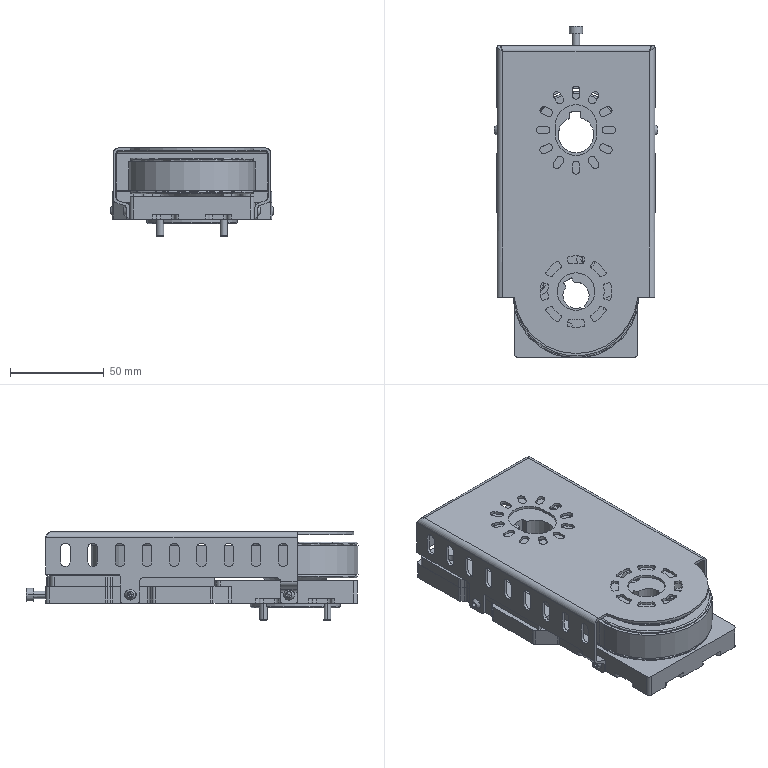Part | SolidWorks | features MoveFace 4, BaseBody 3, ICE 2 | 3 solids | 1596 faces | box 87.3 x 177.09 x 47 mm | volume 222121 mm3 | cylinder 921 | plane 596 | cone 45 | spline 34 | commonest cylinder face diameters 0.8 x274 2.98 x146 4 x108 63.7 x66 5 x54 2 x48